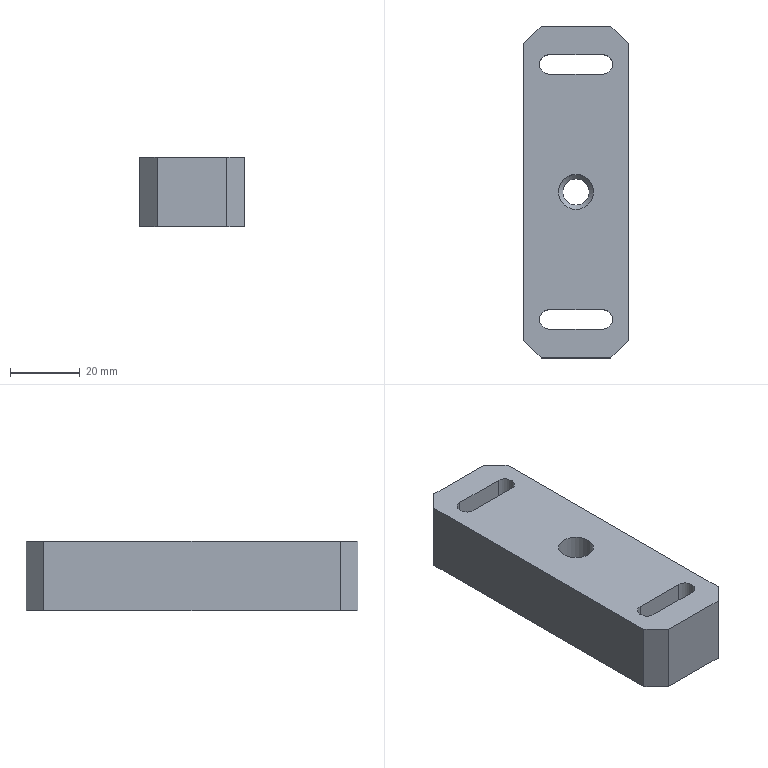Part | NX | features solid 2 | 1 solid | 24 faces | box 30 x 95 x 20 mm | volume 50222 mm3 | plane 14 | cylinder 7 | cone 3 | commonest cylinder face diameters 5.5 x4 10 x2 7.5 x1
STEP:
#1=CARTESIAN_POINT('',(35.,-482.5,-15.));
#2=VERTEX_POINT('',#1);
#3=CARTESIAN_POINT('',(15.,-482.5,-15.));
#4=VERTEX_POINT('',#3);
#5=CARTESIAN_POINT('',(40.,-482.5,-15.));
#6=DIRECTION('',(-1.,0.,0.));
#7=VECTOR('',#6,1000.);
#8=LINE('',#5,#7);
#9=EDGE_CURVE('',#2,#4,#8,.T.);
#10=ORIENTED_EDGE('',*,*,#9,.F.);
#11=CARTESIAN_POINT('',(40.,-477.5,-15.));
#12=VERTEX_POINT('',#11);
#13=CARTESIAN_POINT('',(35.,-482.5,-15.));
#14=DIRECTION('',(-0.7071,-0.7071,0.));
#15=VECTOR('',#14,1000.);
#16=LINE('',#13,#15);
#17=EDGE_CURVE('',#2,#12,#16,.F.);
#18=ORIENTED_EDGE('',*,*,#17,.T.);
#19=CARTESIAN_POINT('',(40.,-392.5,-15.));
#20=VERTEX_POINT('',#19);
#21=CARTESIAN_POINT('',(40.,-387.5,-15.));
#22=DIRECTION('',(0.,-1.,0.));
#23=VECTOR('',#22,1000.);
#24=LINE('',#21,#23);
#25=EDGE_CURVE('',#20,#12,#24,.T.);
#26=ORIENTED_EDGE('',*,*,#25,.F.);
#27=CARTESIAN_POINT('',(35.,-387.5,-15.));
#28=VERTEX_POINT('',#27);
#29=CARTESIAN_POINT('',(40.,-392.5,-15.));
#30=DIRECTION('',(0.7071,-0.7071,0.));
#31=VECTOR('',#30,1000.);
#32=LINE('',#29,#31);
#33=EDGE_CURVE('',#20,#28,#32,.F.);
#34=ORIENTED_EDGE('',*,*,#33,.T.);
#35=CARTESIAN_POINT('',(15.,-387.5,-15.));
#36=VERTEX_POINT('',#35);
#37=CARTESIAN_POINT('',(10.,-387.5,-15.));
#38=DIRECTION('',(1.,0.,0.));
#39=VECTOR('',#38,1000.);
#40=LINE('',#37,#39);
#41=EDGE_CURVE('',#36,#28,#40,.T.);
#42=ORIENTED_EDGE('',*,*,#41,.F.);
#43=CARTESIAN_POINT('',(10.,-392.5,-15.));
#44=VERTEX_POINT('',#43);
#45=CARTESIAN_POINT('',(15.,-387.5,-15.));
#46=DIRECTION('',(0.7071,0.7071,0.));
#47=VECTOR('',#46,1000.);
#48=LINE('',#45,#47);
#49=EDGE_CURVE('',#36,#44,#48,.F.);
#50=ORIENTED_EDGE('',*,*,#49,.T.);
#51=CARTESIAN_POINT('',(10.,-477.5,-15.));
#52=VERTEX_POINT('',#51);
#53=CARTESIAN_POINT('',(10.,-482.5,-15.));
#54=DIRECTION('',(0.,1.,0.));
#55=VECTOR('',#54,1000.);
#56=LINE('',#53,#55);
#57=EDGE_CURVE('',#52,#44,#56,.T.);
#58=ORIENTED_EDGE('',*,*,#57,.F.);
#59=CARTESIAN_POINT('',(10.,-477.5,-15.));
#60=DIRECTION('',(-0.7071,0.7071,0.));
#61=VECTOR('',#60,1000.);
#62=LINE('',#59,#61);
#63=EDGE_CURVE('',#52,#4,#62,.F.);
#64=ORIENTED_EDGE('',*,*,#63,.T.);
#65=EDGE_LOOP('',(#10,#18,#26,#34,#42,#50,#58,#64));
#66=FACE_BOUND('',#65,.T.);
#67=CARTESIAN_POINT('',(17.25,-468.75,-15.));
#68=VERTEX_POINT('',#67);
#69=CARTESIAN_POINT('',(17.25,-474.25,-15.));
#70=VERTEX_POINT('',#69);
#71=CARTESIAN_POINT('',(17.25,-471.5,-15.));
#72=DIRECTION('',(0.,0.,1.));
#73=DIRECTION('',(0.,1.,0.));
#74=AXIS2_PLACEMENT_3D('',#71,#72,#73);
#75=CIRCLE('',#74,2.75);
#76=EDGE_CURVE('',#68,#70,#75,.T.);
#77=ORIENTED_EDGE('',*,*,#76,.F.);
#78=CARTESIAN_POINT('',(32.75,-468.75,-15.));
#79=VERTEX_POINT('',#78);
#80=CARTESIAN_POINT('',(25.,-468.75,-15.));
#81=DIRECTION('',(1.,0.,0.));
#82=VECTOR('',#81,1000.);
#83=LINE('',#80,#82);
#84=EDGE_CURVE('',#68,#79,#83,.T.);
#85=ORIENTED_EDGE('',*,*,#84,.T.);
#86=CARTESIAN_POINT('',(32.75,-474.25,-15.));
#87=VERTEX_POINT('',#86);
#88=CARTESIAN_POINT('',(32.75,-471.5,-15.));
#89=DIRECTION('',(0.,0.,1.));
#90=DIRECTION('',(0.,1.,0.));
#91=AXIS2_PLACEMENT_3D('',#88,#89,#90);
#92=CIRCLE('',#91,2.75);
#93=EDGE_CURVE('',#87,#79,#92,.T.);
#94=ORIENTED_EDGE('',*,*,#93,.F.);
#95=CARTESIAN_POINT('',(25.,-474.25,-15.));
#96=DIRECTION('',(1.,0.,0.));
#97=VECTOR('',#96,1000.);
#98=LINE('',#95,#97);
#99=EDGE_CURVE('',#70,#87,#98,.T.);
#100=ORIENTED_EDGE('',*,*,#99,.F.);
#101=EDGE_LOOP('',(#77,#85,#94,#100));
#102=FACE_BOUND('',#101,.T.);
#103=CARTESIAN_POINT('',(17.25,-395.75,-15.));
#104=VERTEX_POINT('',#103);
#105=CARTESIAN_POINT('',(17.25,-401.25,-15.));
#106=VERTEX_POINT('',#105);
#107=CARTESIAN_POINT('',(17.25,-398.5,-15.));
#108=DIRECTION('',(0.,0.,1.));
#109=DIRECTION('',(0.,1.,0.));
#110=AXIS2_PLACEMENT_3D('',#107,#108,#109);
#111=CIRCLE('',#110,2.75);
#112=EDGE_CURVE('',#104,#106,#111,.T.);
#113=ORIENTED_EDGE('',*,*,#112,.F.);
#114=CARTESIAN_POINT('',(32.75,-395.75,-15.));
#115=VERTEX_POINT('',#114);
#116=CARTESIAN_POINT('',(25.,-395.75,-15.));
#117=DIRECTION('',(1.,0.,0.));
#118=VECTOR('',#117,1000.);
#119=LINE('',#116,#118);
#120=EDGE_CURVE('',#104,#115,#119,.T.);
#121=ORIENTED_EDGE('',*,*,#120,.T.);
#122=CARTESIAN_POINT('',(32.75,-401.25,-15.));
#123=VERTEX_POINT('',#122);
#124=CARTESIAN_POINT('',(32.75,-398.5,-15.));
#125=DIRECTION('',(0.,0.,1.));
#126=DIRECTION('',(0.,1.,0.));
#127=AXIS2_PLACEMENT_3D('',#124,#125,#126);
#128=CIRCLE('',#127,2.75);
#129=EDGE_CURVE('',#123,#115,#128,.T.);
#130=ORIENTED_EDGE('',*,*,#129,.F.);
#131=CARTESIAN_POINT('',(25.,-401.25,-15.));
#132=DIRECTION('',(1.,0.,0.));
#133=VECTOR('',#132,1000.);
#134=LINE('',#131,#133);
#135=EDGE_CURVE('',#106,#123,#134,.T.);
#136=ORIENTED_EDGE('',*,*,#135,.F.);
#137=EDGE_LOOP('',(#113,#121,#130,#136));
#138=FACE_BOUND('',#137,.T.);
#139=CARTESIAN_POINT('',(25.,-440.,-15.));
#140=VERTEX_POINT('',#139);
#141=CARTESIAN_POINT('',(25.,-435.,-15.));
#142=DIRECTION('',(0.,0.,-1.));
#143=DIRECTION('',(0.,-1.,0.));
#144=AXIS2_PLACEMENT_3D('',#141,#142,#143);
#145=CIRCLE('',#144,5.);
#146=EDGE_CURVE('',#140,#140,#145,.T.);
#147=ORIENTED_EDGE('',*,*,#146,.T.);
#148=EDGE_LOOP('',(#147));
#149=FACE_BOUND('',#148,.T.);
#150=CARTESIAN_POINT('',(10.,-482.5,-15.));
#151=DIRECTION('',(0.,0.,-1.));
#152=DIRECTION('',(0.,-1.,0.));
#153=AXIS2_PLACEMENT_3D('',#150,#151,#152);
#154=PLANE('',#153);
#155=ADVANCED_FACE('',(#66,#102,#138,#149),#154,.F.);
#156=CARTESIAN_POINT('',(35.,-482.5,-35.));
#157=VERTEX_POINT('',#156);
#158=CARTESIAN_POINT('',(15.,-482.5,-35.));
#159=VERTEX_POINT('',#158);
#160=CARTESIAN_POINT('',(40.,-482.5,-35.));
#161=DIRECTION('',(-1.,0.,0.));
#162=VECTOR('',#161,1000.);
#163=LINE('',#160,#162);
#164=EDGE_CURVE('',#157,#159,#163,.T.);
#165=ORIENTED_EDGE('',*,*,#164,.F.);
#166=CARTESIAN_POINT('',(35.,-482.5,-35.));
#167=DIRECTION('',(0.,0.,1.));
#168=VECTOR('',#167,1000.);
#169=LINE('',#166,#168);
#170=EDGE_CURVE('',#157,#2,#169,.T.);
#171=ORIENTED_EDGE('',*,*,#170,.T.);
#172=ORIENTED_EDGE('',*,*,#9,.T.);
#173=CARTESIAN_POINT('',(15.,-482.5,-35.));
#174=DIRECTION('',(0.,0.,-1.));
#175=VECTOR('',#174,1000.);
#176=LINE('',#173,#175);
#177=EDGE_CURVE('',#4,#159,#176,.T.);
#178=ORIENTED_EDGE('',*,*,#177,.T.);
#179=EDGE_LOOP('',(#165,#171,#172,#178));
#180=FACE_BOUND('',#179,.T.);
#181=CARTESIAN_POINT('',(40.,-482.5,-35.));
#182=DIRECTION('',(0.,1.,0.));
#183=DIRECTION('',(0.,0.,-1.));
#184=AXIS2_PLACEMENT_3D('',#181,#182,#183);
#185=PLANE('',#184);
#186=ADVANCED_FACE('',(#180),#185,.F.);
#187=CARTESIAN_POINT('',(10.,-477.5,-35.));
#188=VERTEX_POINT('',#187);
#189=CARTESIAN_POINT('',(10.,-392.5,-35.));
#190=VERTEX_POINT('',#189);
#191=CARTESIAN_POINT('',(10.,-482.5,-35.));
#192=DIRECTION('',(0.,1.,0.));
#193=VECTOR('',#192,1000.);
#194=LINE('',#191,#193);
#195=EDGE_CURVE('',#188,#190,#194,.T.);
#196=ORIENTED_EDGE('',*,*,#195,.F.);
#197=CARTESIAN_POINT('',(10.,-477.5,-35.));
#198=DIRECTION('',(0.,0.,1.));
#199=VECTOR('',#198,1000.);
#200=LINE('',#197,#199);
#201=EDGE_CURVE('',#188,#52,#200,.T.);
#202=ORIENTED_EDGE('',*,*,#201,.T.);
#203=ORIENTED_EDGE('',*,*,#57,.T.);
#204=CARTESIAN_POINT('',(10.,-392.5,-35.));
#205=DIRECTION('',(0.,0.,-1.));
#206=VECTOR('',#205,1000.);
#207=LINE('',#204,#206);
#208=EDGE_CURVE('',#44,#190,#207,.T.);
#209=ORIENTED_EDGE('',*,*,#208,.T.);
#210=EDGE_LOOP('',(#196,#202,#203,#209));
#211=FACE_BOUND('',#210,.T.);
#212=CARTESIAN_POINT('',(10.,-482.5,-35.));
#213=DIRECTION('',(1.,0.,0.));
#214=DIRECTION('',(0.,0.,1.));
#215=AXIS2_PLACEMENT_3D('',#212,#213,#214);
#216=PLANE('',#215);
#217=ADVANCED_FACE('',(#211),#216,.F.);
#218=CARTESIAN_POINT('',(15.,-387.5,-35.));
#219=VERTEX_POINT('',#218);
#220=CARTESIAN_POINT('',(35.,-387.5,-35.));
#221=VERTEX_POINT('',#220);
#222=CARTESIAN_POINT('',(10.,-387.5,-35.));
#223=DIRECTION('',(1.,0.,0.));
#224=VECTOR('',#223,1000.);
#225=LINE('',#222,#224);
#226=EDGE_CURVE('',#219,#221,#225,.T.);
#227=ORIENTED_EDGE('',*,*,#226,.F.);
#228=CARTESIAN_POINT('',(15.,-387.5,-35.));
#229=DIRECTION('',(0.,0.,1.));
#230=VECTOR('',#229,1000.);
#231=LINE('',#228,#230);
#232=EDGE_CURVE('',#219,#36,#231,.T.);
#233=ORIENTED_EDGE('',*,*,#232,.T.);
#234=ORIENTED_EDGE('',*,*,#41,.T.);
#235=CARTESIAN_POINT('',(35.,-387.5,-35.));
#236=DIRECTION('',(0.,0.,-1.));
#237=VECTOR('',#236,1000.);
#238=LINE('',#235,#237);
#239=EDGE_CURVE('',#28,#221,#238,.T.);
#240=ORIENTED_EDGE('',*,*,#239,.T.);
#241=EDGE_LOOP('',(#227,#233,#234,#240));
#242=FACE_BOUND('',#241,.T.);
#243=CARTESIAN_POINT('',(10.,-387.5,-35.));
#244=DIRECTION('',(0.,-1.,0.));
#245=DIRECTION('',(0.,0.,1.));
#246=AXIS2_PLACEMENT_3D('',#243,#244,#245);
#247=PLANE('',#246);
#248=ADVANCED_FACE('',(#242),#247,.F.);
#249=ORIENTED_EDGE('',*,*,#25,.T.);
#250=CARTESIAN_POINT('',(40.,-477.5,-35.));
#251=VERTEX_POINT('',#250);
#252=CARTESIAN_POINT('',(40.,-477.5,-35.));
#253=DIRECTION('',(0.,0.,-1.));
#254=VECTOR('',#253,1000.);
#255=LINE('',#252,#254);
#256=EDGE_CURVE('',#12,#251,#255,.T.);
#257=ORIENTED_EDGE('',*,*,#256,.T.);
#258=CARTESIAN_POINT('',(40.,-392.5,-35.));
#259=VERTEX_POINT('',#258);
#260=CARTESIAN_POINT('',(40.,-387.5,-35.));
#261=DIRECTION('',(0.,-1.,0.));
#262=VECTOR('',#261,1000.);
#263=LINE('',#260,#262);
#264=EDGE_CURVE('',#259,#251,#263,.T.);
#265=ORIENTED_EDGE('',*,*,#264,.F.);
#266=CARTESIAN_POINT('',(40.,-392.5,-35.));
#267=DIRECTION('',(0.,0.,1.));
#268=VECTOR('',#267,1000.);
#269=LINE('',#266,#268);
#270=EDGE_CURVE('',#259,#20,#269,.T.);
#271=ORIENTED_EDGE('',*,*,#270,.T.);
#272=EDGE_LOOP('',(#249,#257,#265,#271));
#273=FACE_BOUND('',#272,.T.);
#274=CARTESIAN_POINT('',(40.,-387.5,-35.));
#275=DIRECTION('',(-1.,0.,0.));
#276=DIRECTION('',(0.,0.,-1.));
#277=AXIS2_PLACEMENT_3D('',#274,#275,#276);
#278=PLANE('',#277);
#279=ADVANCED_FACE('',(#273),#278,.F.);
#280=CARTESIAN_POINT('',(25.,-438.75,-35.));
#281=VERTEX_POINT('',#280);
#282=CARTESIAN_POINT('',(25.,-435.,-35.));
#283=DIRECTION('',(0.,0.,-1.));
#284=DIRECTION('',(0.,-1.,0.));
#285=AXIS2_PLACEMENT_3D('',#282,#283,#284);
#286=CIRCLE('',#285,3.75);
#287=EDGE_CURVE('',#281,#281,#286,.T.);
#288=ORIENTED_EDGE('',*,*,#287,.F.);
#289=EDGE_LOOP('',(#288));
#290=FACE_BOUND('',#289,.T.);
#291=CARTESIAN_POINT('',(17.25,-395.75,-35.));
#292=VERTEX_POINT('',#291);
#293=CARTESIAN_POINT('',(32.75,-395.75,-35.));
#294=VERTEX_POINT('',#293);
#295=CARTESIAN_POINT('',(10.,-395.75,-35.));
#296=DIRECTION('',(1.,0.,0.));
#297=VECTOR('',#296,1000.);
#298=LINE('',#295,#297);
#299=EDGE_CURVE('',#292,#294,#298,.T.);
#300=ORIENTED_EDGE('',*,*,#299,.F.);
#301=CARTESIAN_POINT('',(17.25,-401.25,-35.));
#302=VERTEX_POINT('',#301);
#303=CARTESIAN_POINT('',(17.25,-398.5,-35.));
#304=DIRECTION('',(0.,0.,-1.));
#305=DIRECTION('',(0.,-1.,0.));
#306=AXIS2_PLACEMENT_3D('',#303,#304,#305);
#307=CIRCLE('',#306,2.75);
#308=EDGE_CURVE('',#302,#292,#307,.T.);
#309=ORIENTED_EDGE('',*,*,#308,.F.);
#310=CARTESIAN_POINT('',(32.75,-401.25,-35.));
#311=VERTEX_POINT('',#310);
#312=CARTESIAN_POINT('',(10.,-401.25,-35.));
#313=DIRECTION('',(-1.,0.,0.));
#314=VECTOR('',#313,1000.);
#315=LINE('',#312,#314);
#316=EDGE_CURVE('',#311,#302,#315,.T.);
#317=ORIENTED_EDGE('',*,*,#316,.F.);
#318=CARTESIAN_POINT('',(32.75,-398.5,-35.));
#319=DIRECTION('',(0.,0.,-1.));
#320=DIRECTION('',(0.,-1.,0.));
#321=AXIS2_PLACEMENT_3D('',#318,#319,#320);
#322=CIRCLE('',#321,2.75);
#323=EDGE_CURVE('',#294,#311,#322,.T.);
#324=ORIENTED_EDGE('',*,*,#323,.F.);
#325=EDGE_LOOP('',(#300,#309,#317,#324));
#326=FACE_BOUND('',#325,.T.);
#327=CARTESIAN_POINT('',(17.25,-468.75,-35.));
#328=VERTEX_POINT('',#327);
#329=CARTESIAN_POINT('',(32.75,-468.75,-35.));
#330=VERTEX_POINT('',#329);
#331=CARTESIAN_POINT('',(10.,-468.75,-35.));
#332=DIRECTION('',(1.,0.,0.));
#333=VECTOR('',#332,1000.);
#334=LINE('',#331,#333);
#335=EDGE_CURVE('',#328,#330,#334,.T.);
#336=ORIENTED_EDGE('',*,*,#335,.F.);
#337=CARTESIAN_POINT('',(17.25,-474.25,-35.));
#338=VERTEX_POINT('',#337);
#339=CARTESIAN_POINT('',(17.25,-471.5,-35.));
#340=DIRECTION('',(0.,0.,-1.));
#341=DIRECTION('',(0.,-1.,0.));
#342=AXIS2_PLACEMENT_3D('',#339,#340,#341);
#343=CIRCLE('',#342,2.75);
#344=EDGE_CURVE('',#338,#328,#343,.T.);
#345=ORIENTED_EDGE('',*,*,#344,.F.);
#346=CARTESIAN_POINT('',(32.75,-474.25,-35.));
#347=VERTEX_POINT('',#346);
#348=CARTESIAN_POINT('',(10.,-474.25,-35.));
#349=DIRECTION('',(-1.,0.,0.));
#350=VECTOR('',#349,1000.);
#351=LINE('',#348,#350);
#352=EDGE_CURVE('',#347,#338,#351,.T.);
#353=ORIENTED_EDGE('',*,*,#352,.F.);
#354=CARTESIAN_POINT('',(32.75,-471.5,-35.));
#355=DIRECTION('',(0.,0.,-1.));
#356=DIRECTION('',(0.,-1.,0.));
#357=AXIS2_PLACEMENT_3D('',#354,#355,#356);
#358=CIRCLE('',#357,2.75);
#359=EDGE_CURVE('',#330,#347,#358,.T.);
#360=ORIENTED_EDGE('',*,*,#359,.F.);
#361=EDGE_LOOP('',(#336,#345,#353,#360));
#362=FACE_BOUND('',#361,.T.);
#363=ORIENTED_EDGE('',*,*,#264,.T.);
#364=CARTESIAN_POINT('',(22.5,-495.,-35.));
#365=DIRECTION('',(0.7071,0.7071,0.));
#366=VECTOR('',#365,1000.);
#367=LINE('',#364,#366);
#368=EDGE_CURVE('',#251,#157,#367,.F.);
#369=ORIENTED_EDGE('',*,*,#368,.T.);
#370=ORIENTED_EDGE('',*,*,#164,.T.);
#371=CARTESIAN_POINT('',(12.5,-480.,-35.));
#372=DIRECTION('',(0.7071,-0.7071,0.));
#373=VECTOR('',#372,1000.);
#374=LINE('',#371,#373);
#375=EDGE_CURVE('',#159,#188,#374,.F.);
#376=ORIENTED_EDGE('',*,*,#375,.T.);
#377=ORIENTED_EDGE('',*,*,#195,.T.);
#378=CARTESIAN_POINT('',(-35.,-437.5,-35.));
#379=DIRECTION('',(-0.7071,-0.7071,0.));
#380=VECTOR('',#379,1000.);
#381=LINE('',#378,#380);
#382=EDGE_CURVE('',#190,#219,#381,.F.);
#383=ORIENTED_EDGE('',*,*,#382,.T.);
#384=ORIENTED_EDGE('',*,*,#226,.T.);
#385=CARTESIAN_POINT('',(70.,-422.5,-35.));
#386=DIRECTION('',(-0.7071,0.7071,0.));
#387=VECTOR('',#386,1000.);
#388=LINE('',#385,#387);
#389=EDGE_CURVE('',#221,#259,#388,.F.);
#390=ORIENTED_EDGE('',*,*,#389,.T.);
#391=EDGE_LOOP('',(#363,#369,#370,#376,#377,#383,#384,#390));
#392=FACE_BOUND('',#391,.T.);
#393=CARTESIAN_POINT('',(10.,-482.5,-35.));
#394=DIRECTION('',(0.,0.,-1.));
#395=DIRECTION('',(0.,-1.,0.));
#396=AXIS2_PLACEMENT_3D('',#393,#394,#395);
#397=PLANE('',#396);
#398=ADVANCED_FACE('',(#290,#326,#362,#392),#397,.T.);
#399=ORIENTED_EDGE('',*,*,#335,.T.);
#400=CARTESIAN_POINT('',(32.75,-468.75,-15.));
#401=DIRECTION('',(0.,0.,1.));
#402=VECTOR('',#401,1000.);
#403=LINE('',#400,#402);
#404=EDGE_CURVE('',#330,#79,#403,.T.);
#405=ORIENTED_EDGE('',*,*,#404,.T.);
#406=ORIENTED_EDGE('',*,*,#84,.F.);
#407=CARTESIAN_POINT('',(17.25,-468.75,-15.));
#408=DIRECTION('',(0.,0.,1.));
#409=VECTOR('',#408,1000.);
#410=LINE('',#407,#409);
#411=EDGE_CURVE('',#328,#68,#410,.T.);
#412=ORIENTED_EDGE('',*,*,#411,.F.);
#413=EDGE_LOOP('',(#399,#405,#406,#412));
#414=FACE_BOUND('',#413,.T.);
#415=CARTESIAN_POINT('',(25.,-468.75,-15.));
#416=DIRECTION('',(0.,1.,0.));
#417=DIRECTION('',(0.,0.,-1.));
#418=AXIS2_PLACEMENT_3D('',#415,#416,#417);
#419=PLANE('',#418);
#420=ADVANCED_FACE('',(#414),#419,.F.);
#421=ORIENTED_EDGE('',*,*,#344,.T.);
#422=ORIENTED_EDGE('',*,*,#411,.T.);
#423=ORIENTED_EDGE('',*,*,#76,.T.);
#424=CARTESIAN_POINT('',(17.25,-474.25,-15.));
#425=DIRECTION('',(0.,0.,1.));
#426=VECTOR('',#425,1000.);
#427=LINE('',#424,#426);
#428=EDGE_CURVE('',#338,#70,#427,.T.);
#429=ORIENTED_EDGE('',*,*,#428,.F.);
#430=EDGE_LOOP('',(#421,#422,#423,#429));
#431=FACE_BOUND('',#430,.T.);
#432=CARTESIAN_POINT('',(17.25,-471.5,-15.));
#433=DIRECTION('',(0.,0.,1.));
#434=DIRECTION('',(0.,1.,0.));
#435=AXIS2_PLACEMENT_3D('',#432,#433,#434);
#436=CYLINDRICAL_SURFACE('',#435,2.75);
#437=ADVANCED_FACE('',(#431),#436,.F.);
#438=ORIENTED_EDGE('',*,*,#352,.T.);
#439=ORIENTED_EDGE('',*,*,#428,.T.);
#440=ORIENTED_EDGE('',*,*,#99,.T.);
#441=CARTESIAN_POINT('',(32.75,-474.25,-15.));
#442=DIRECTION('',(0.,0.,1.));
#443=VECTOR('',#442,1000.);
#444=LINE('',#441,#443);
#445=EDGE_CURVE('',#347,#87,#444,.T.);
#446=ORIENTED_EDGE('',*,*,#445,.F.);
#447=EDGE_LOOP('',(#438,#439,#440,#446));
#448=FACE_BOUND('',#447,.T.);
#449=CARTESIAN_POINT('',(25.,-474.25,-15.));
#450=DIRECTION('',(0.,-1.,0.));
#451=DIRECTION('',(0.,0.,1.));
#452=AXIS2_PLACEMENT_3D('',#449,#450,#451);
#453=PLANE('',#452);
#454=ADVANCED_FACE('',(#448),#453,.F.);
#455=ORIENTED_EDGE('',*,*,#359,.T.);
#456=ORIENTED_EDGE('',*,*,#445,.T.);
#457=ORIENTED_EDGE('',*,*,#93,.T.);
#458=ORIENTED_EDGE('',*,*,#404,.F.);
#459=EDGE_LOOP('',(#455,#456,#457,#458));
#460=FACE_BOUND('',#459,.T.);
#461=CARTESIAN_POINT('',(32.75,-471.5,-15.));
#462=DIRECTION('',(0.,0.,1.));
#463=DIRECTION('',(0.,1.,0.));
#464=AXIS2_PLACEMENT_3D('',#461,#462,#463);
#465=CYLINDRICAL_SURFACE('',#464,2.75);
#466=ADVANCED_FACE('',(#460),#465,.F.);
#467=ORIENTED_EDGE('',*,*,#299,.T.);
#468=CARTESIAN_POINT('',(32.75,-395.75,-15.));
#469=DIRECTION('',(0.,0.,1.));
#470=VECTOR('',#469,1000.);
#471=LINE('',#468,#470);
#472=EDGE_CURVE('',#294,#115,#471,.T.);
#473=ORIENTED_EDGE('',*,*,#472,.T.);
#474=ORIENTED_EDGE('',*,*,#120,.F.);
#475=CARTESIAN_POINT('',(17.25,-395.75,-15.));
#476=DIRECTION('',(0.,0.,1.));
#477=VECTOR('',#476,1000.);
#478=LINE('',#475,#477);
#479=EDGE_CURVE('',#292,#104,#478,.T.);
#480=ORIENTED_EDGE('',*,*,#479,.F.);
#481=EDGE_LOOP('',(#467,#473,#474,#480));
#482=FACE_BOUND('',#481,.T.);
#483=CARTESIAN_POINT('',(25.,-395.75,-15.));
#484=DIRECTION('',(0.,1.,0.));
#485=DIRECTION('',(0.,0.,-1.));
#486=AXIS2_PLACEMENT_3D('',#483,#484,#485);
#487=PLANE('',#486);
#488=ADVANCED_FACE('',(#482),#487,.F.);
#489=ORIENTED_EDGE('',*,*,#308,.T.);
#490=ORIENTED_EDGE('',*,*,#479,.T.);
#491=ORIENTED_EDGE('',*,*,#112,.T.);
#492=CARTESIAN_POINT('',(17.25,-401.25,-15.));
#493=DIRECTION('',(0.,0.,1.));
#494=VECTOR('',#493,1000.);
#495=LINE('',#492,#494);
#496=EDGE_CURVE('',#302,#106,#495,.T.);
#497=ORIENTED_EDGE('',*,*,#496,.F.);
#498=EDGE_LOOP('',(#489,#490,#491,#497));
#499=FACE_BOUND('',#498,.T.);
#500=CARTESIAN_POINT('',(17.25,-398.5,-15.));
#501=DIRECTION('',(0.,0.,1.));
#502=DIRECTION('',(0.,1.,0.));
#503=AXIS2_PLACEMENT_3D('',#500,#501,#502);
#504=CYLINDRICAL_SURFACE('',#503,2.75);
#505=ADVANCED_FACE('',(#499),#504,.F.);
#506=ORIENTED_EDGE('',*,*,#316,.T.);
#507=ORIENTED_EDGE('',*,*,#496,.T.);
#508=ORIENTED_EDGE('',*,*,#135,.T.);
#509=CARTESIAN_POINT('',(32.75,-401.25,-15.));
#510=DIRECTION('',(0.,0.,1.));
#511=VECTOR('',#510,1000.);
#512=LINE('',#509,#511);
#513=EDGE_CURVE('',#311,#123,#512,.T.);
#514=ORIENTED_EDGE('',*,*,#513,.F.);
#515=EDGE_LOOP('',(#506,#507,#508,#514));
#516=FACE_BOUND('',#515,.T.);
#517=CARTESIAN_POINT('',(25.,-401.25,-15.));
#518=DIRECTION('',(0.,-1.,0.));
#519=DIRECTION('',(0.,0.,1.));
#520=AXIS2_PLACEMENT_3D('',#517,#518,#519);
#521=PLANE('',#520);
#522=ADVANCED_FACE('',(#516),#521,.F.);
#523=ORIENTED_EDGE('',*,*,#323,.T.);
#524=ORIENTED_EDGE('',*,*,#513,.T.);
#525=ORIENTED_EDGE('',*,*,#129,.T.);
#526=ORIENTED_EDGE('',*,*,#472,.F.);
#527=EDGE_LOOP('',(#523,#524,#525,#526));
#528=FACE_BOUND('',#527,.T.);
#529=CARTESIAN_POINT('',(32.75,-398.5,-15.));
#530=DIRECTION('',(0.,0.,1.));
#531=DIRECTION('',(0.,1.,0.));
#532=AXIS2_PLACEMENT_3D('',#529,#530,#531);
#533=CYLINDRICAL_SURFACE('',#532,2.75);
#534=ADVANCED_FACE('',(#528),#533,.F.);
#535=ORIENTED_EDGE('',*,*,#389,.F.);
#536=ORIENTED_EDGE('',*,*,#239,.F.);
#537=ORIENTED_EDGE('',*,*,#33,.F.);
#538=ORIENTED_EDGE('',*,*,#270,.F.);
#539=EDGE_LOOP('',(#535,#536,#537,#538));
#540=FACE_BOUND('',#539,.T.);
#541=CARTESIAN_POINT('',(40.,-392.5,-35.));
#542=DIRECTION('',(-0.7071,-0.7071,0.));
#543=DIRECTION('',(-0.7071,0.7071,0.));
#544=AXIS2_PLACEMENT_3D('',#541,#542,#543);
#545=PLANE('',#544);
#546=ADVANCED_FACE('',(#540),#545,.F.);
#547=ORIENTED_EDGE('',*,*,#368,.F.);
#548=ORIENTED_EDGE('',*,*,#256,.F.);
#549=ORIENTED_EDGE('',*,*,#17,.F.);
#550=ORIENTED_EDGE('',*,*,#170,.F.);
#551=EDGE_LOOP('',(#547,#548,#549,#550));
#552=FACE_BOUND('',#551,.T.);
#553=CARTESIAN_POINT('',(35.,-482.5,-35.));
#554=DIRECTION('',(-0.7071,0.7071,0.));
#555=DIRECTION('',(0.7071,0.7071,0.));
#556=AXIS2_PLACEMENT_3D('',#553,#554,#555);
#557=PLANE('',#556);
#558=ADVANCED_FACE('',(#552),#557,.F.);
#559=ORIENTED_EDGE('',*,*,#375,.F.);
#560=ORIENTED_EDGE('',*,*,#177,.F.);
#561=ORIENTED_EDGE('',*,*,#63,.F.);
#562=ORIENTED_EDGE('',*,*,#201,.F.);
#563=EDGE_LOOP('',(#559,#560,#561,#562));
#564=FACE_BOUND('',#563,.T.);
#565=CARTESIAN_POINT('',(10.,-477.5,-35.));
#566=DIRECTION('',(0.7071,0.7071,0.));
#567=DIRECTION('',(0.7071,-0.7071,0.));
#568=AXIS2_PLACEMENT_3D('',#565,#566,#567);
#569=PLANE('',#568);
#570=ADVANCED_FACE('',(#564),#569,.F.);
#571=ORIENTED_EDGE('',*,*,#382,.F.);
#572=ORIENTED_EDGE('',*,*,#208,.F.);
#573=ORIENTED_EDGE('',*,*,#49,.F.);
#574=ORIENTED_EDGE('',*,*,#232,.F.);
#575=EDGE_LOOP('',(#571,#572,#573,#574));
#576=FACE_BOUND('',#575,.T.);
#577=CARTESIAN_POINT('',(15.,-387.5,-35.));
#578=DIRECTION('',(0.7071,-0.7071,0.));
#579=DIRECTION('',(-0.7071,-0.7071,0.));
#580=AXIS2_PLACEMENT_3D('',#577,#578,#579);
#581=PLANE('',#580);
#582=ADVANCED_FACE('',(#576),#581,.F.);
#583=CARTESIAN_POINT('',(25.,-440.,-25.5));
#584=VERTEX_POINT('',#583);
#585=CARTESIAN_POINT('',(25.,-435.,-25.5));
#586=DIRECTION('',(0.,0.,-1.));
#587=DIRECTION('',(0.,-1.,0.));
#588=AXIS2_PLACEMENT_3D('',#585,#586,#587);
#589=CIRCLE('',#588,5.);
#590=EDGE_CURVE('',#584,#584,#589,.F.);
#591=ORIENTED_EDGE('',*,*,#590,.F.);
#592=EDGE_LOOP('',(#591));
#593=FACE_BOUND('',#592,.T.);
#594=ORIENTED_EDGE('',*,*,#146,.F.);
#595=EDGE_LOOP('',(#594));
#596=FACE_BOUND('',#595,.T.);
#597=CARTESIAN_POINT('',(25.,-435.,-35.));
#598=DIRECTION('',(0.,0.,1.));
#599=DIRECTION('',(0.,1.,0.));
#600=AXIS2_PLACEMENT_3D('',#597,#598,#599);
#601=CYLINDRICAL_SURFACE('',#600,5.);
#602=ADVANCED_FACE('',(#593,#596),#601,.F.);
#603=CARTESIAN_POINT('',(25.,-440.,-33.75));
#604=VERTEX_POINT('',#603);
#605=CARTESIAN_POINT('',(25.,-435.,-33.75));
#606=DIRECTION('',(0.,0.,-1.));
#607=DIRECTION('',(0.,-1.,0.));
#608=AXIS2_PLACEMENT_3D('',#605,#606,#607);
#609=CIRCLE('',#608,5.);
#610=EDGE_CURVE('',#604,#604,#609,.F.);
#611=ORIENTED_EDGE('',*,*,#610,.F.);
#612=EDGE_LOOP('',(#611));
#613=FACE_BOUND('',#612,.T.);
#614=CARTESIAN_POINT('',(25.,-430.,-30.5));
#615=VERTEX_POINT('',#614);
#616=CARTESIAN_POINT('',(25.,-435.,-30.5));
#617=DIRECTION('',(0.,0.,1.));
#618=DIRECTION('',(0.,1.,0.));
#619=AXIS2_PLACEMENT_3D('',#616,#617,#618);
#620=CIRCLE('',#619,5.);
#621=EDGE_CURVE('',#615,#615,#620,.F.);
#622=ORIENTED_EDGE('',*,*,#621,.F.);
#623=EDGE_LOOP('',(#622));
#624=FACE_BOUND('',#623,.T.);
#625=CARTESIAN_POINT('',(25.,-435.,-35.));
#626=DIRECTION('',(0.,0.,1.));
#627=DIRECTION('',(0.,1.,0.));
#628=AXIS2_PLACEMENT_3D('',#625,#626,#627);
#629=CYLINDRICAL_SURFACE('',#628,5.);
#630=ADVANCED_FACE('',(#613,#624),#629,.F.);
#631=CARTESIAN_POINT('',(25.,-438.75,-29.25));
#632=VERTEX_POINT('',#631);
#633=CARTESIAN_POINT('',(25.,-435.,-29.25));
#634=DIRECTION('',(0.,0.,-1.));
#635=DIRECTION('',(0.,-1.,0.));
#636=AXIS2_PLACEMENT_3D('',#633,#634,#635);
#637=CIRCLE('',#636,3.75);
#638=EDGE_CURVE('',#632,#632,#637,.T.);
#639=ORIENTED_EDGE('',*,*,#638,.T.);
#640=EDGE_LOOP('',(#639));
#641=FACE_BOUND('',#640,.T.);
#642=CARTESIAN_POINT('',(25.,-438.75,-26.75));
#643=VERTEX_POINT('',#642);
#644=CARTESIAN_POINT('',(25.,-435.,-26.75));
#645=DIRECTION('',(0.,0.,-1.));
#646=DIRECTION('',(0.,-1.,0.));
#647=AXIS2_PLACEMENT_3D('',#644,#645,#646);
#648=CIRCLE('',#647,3.75);
#649=EDGE_CURVE('',#643,#643,#648,.T.);
#650=ORIENTED_EDGE('',*,*,#649,.F.);
#651=EDGE_LOOP('',(#650));
#652=FACE_BOUND('',#651,.T.);
#653=CARTESIAN_POINT('',(25.,-435.,-26.75));
#654=DIRECTION('',(0.,0.,-1.));
#655=DIRECTION('',(0.,-1.,0.));
#656=AXIS2_PLACEMENT_3D('',#653,#654,#655);
#657=CYLINDRICAL_SURFACE('',#656,3.75);
#658=ADVANCED_FACE('',(#641,#652),#657,.F.);
#659=ORIENTED_EDGE('',*,*,#638,.F.);
#660=EDGE_LOOP('',(#659));
#661=FACE_BOUND('',#660,.T.);
#662=ORIENTED_EDGE('',*,*,#621,.T.);
#663=EDGE_LOOP('',(#662));
#664=FACE_BOUND('',#663,.T.);
#665=CARTESIAN_POINT('',(25.,-435.,-30.5));
#666=DIRECTION('',(0.,0.,-1.));
#667=DIRECTION('',(0.,-1.,0.));
#668=AXIS2_PLACEMENT_3D('',#665,#666,#667);
#669=CONICAL_SURFACE('',#668,5.,0.7854);
#670=ADVANCED_FACE('',(#661,#664),#669,.F.);
#671=ORIENTED_EDGE('',*,*,#590,.T.);
#672=EDGE_LOOP('',(#671));
#673=FACE_BOUND('',#672,.T.);
#674=ORIENTED_EDGE('',*,*,#649,.T.);
#675=EDGE_LOOP('',(#674));
#676=FACE_BOUND('',#675,.T.);
#677=CARTESIAN_POINT('',(25.,-435.,-26.75));
#678=DIRECTION('',(0.,0.,1.));
#679=DIRECTION('',(0.,1.,0.));
#680=AXIS2_PLACEMENT_3D('',#677,#678,#679);
#681=CONICAL_SURFACE('',#680,3.75,0.7854);
#682=ADVANCED_FACE('',(#673,#676),#681,.F.);
#683=ORIENTED_EDGE('',*,*,#610,.T.);
#684=EDGE_LOOP('',(#683));
#685=FACE_BOUND('',#684,.T.);
#686=ORIENTED_EDGE('',*,*,#287,.T.);
#687=EDGE_LOOP('',(#686));
#688=FACE_BOUND('',#687,.T.);
#689=CARTESIAN_POINT('',(25.,-435.,-35.));
#690=DIRECTION('',(0.,0.,1.));
#691=DIRECTION('',(0.,1.,0.));
#692=AXIS2_PLACEMENT_3D('',#689,#690,#691);
#693=CONICAL_SURFACE('',#692,3.75,0.7854);
#694=ADVANCED_FACE('',(#685,#688),#693,.F.);
#695=CLOSED_SHELL('',(#155,#186,#217,#248,#279,#398,#420,#437,#454,#466,#488,#505,#522,#534,#546,#558,#570,#582,#602,#630,#658,#670,#682,#694));
#696=MANIFOLD_SOLID_BREP('',#695);
#697=(LENGTH_UNIT()NAMED_UNIT(*)SI_UNIT(.MILLI.,.METRE.));
#698=UNCERTAINTY_MEASURE_WITH_UNIT(LENGTH_MEASURE(0.00001),#697,'','');
#699=(NAMED_UNIT(*)PLANE_ANGLE_UNIT()SI_UNIT($,.RADIAN.));
#700=(NAMED_UNIT(*)SI_UNIT($,.STERADIAN.)SOLID_ANGLE_UNIT());
#701=(GEOMETRIC_REPRESENTATION_CONTEXT(3)GLOBAL_UNCERTAINTY_ASSIGNED_CONTEXT((#698))GLOBAL_UNIT_ASSIGNED_CONTEXT((#697,#699,#700))REPRESENTATION_CONTEXT('',''));
#702=ADVANCED_BREP_SHAPE_REPRESENTATION('',(#696),#701);